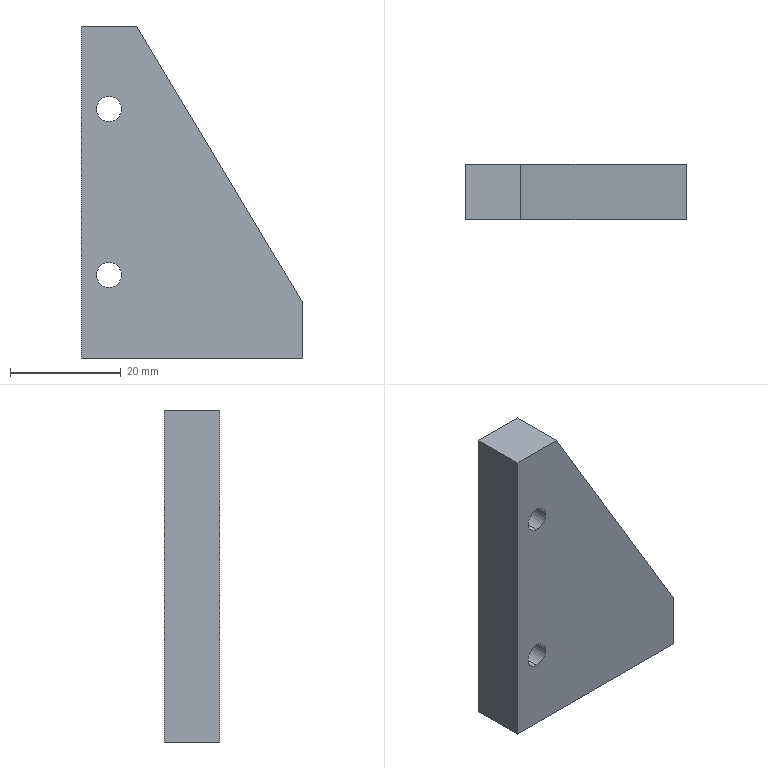Part | STEP file | PN_0023 | 1 solid | 25 faces | box 40 x 10 x 60 mm | volume 15663 mm3 | cylinder 12 | plane 9 | cone 4 | commonest cylinder face diameters 3.3 x4 4.5 x4 8 x4